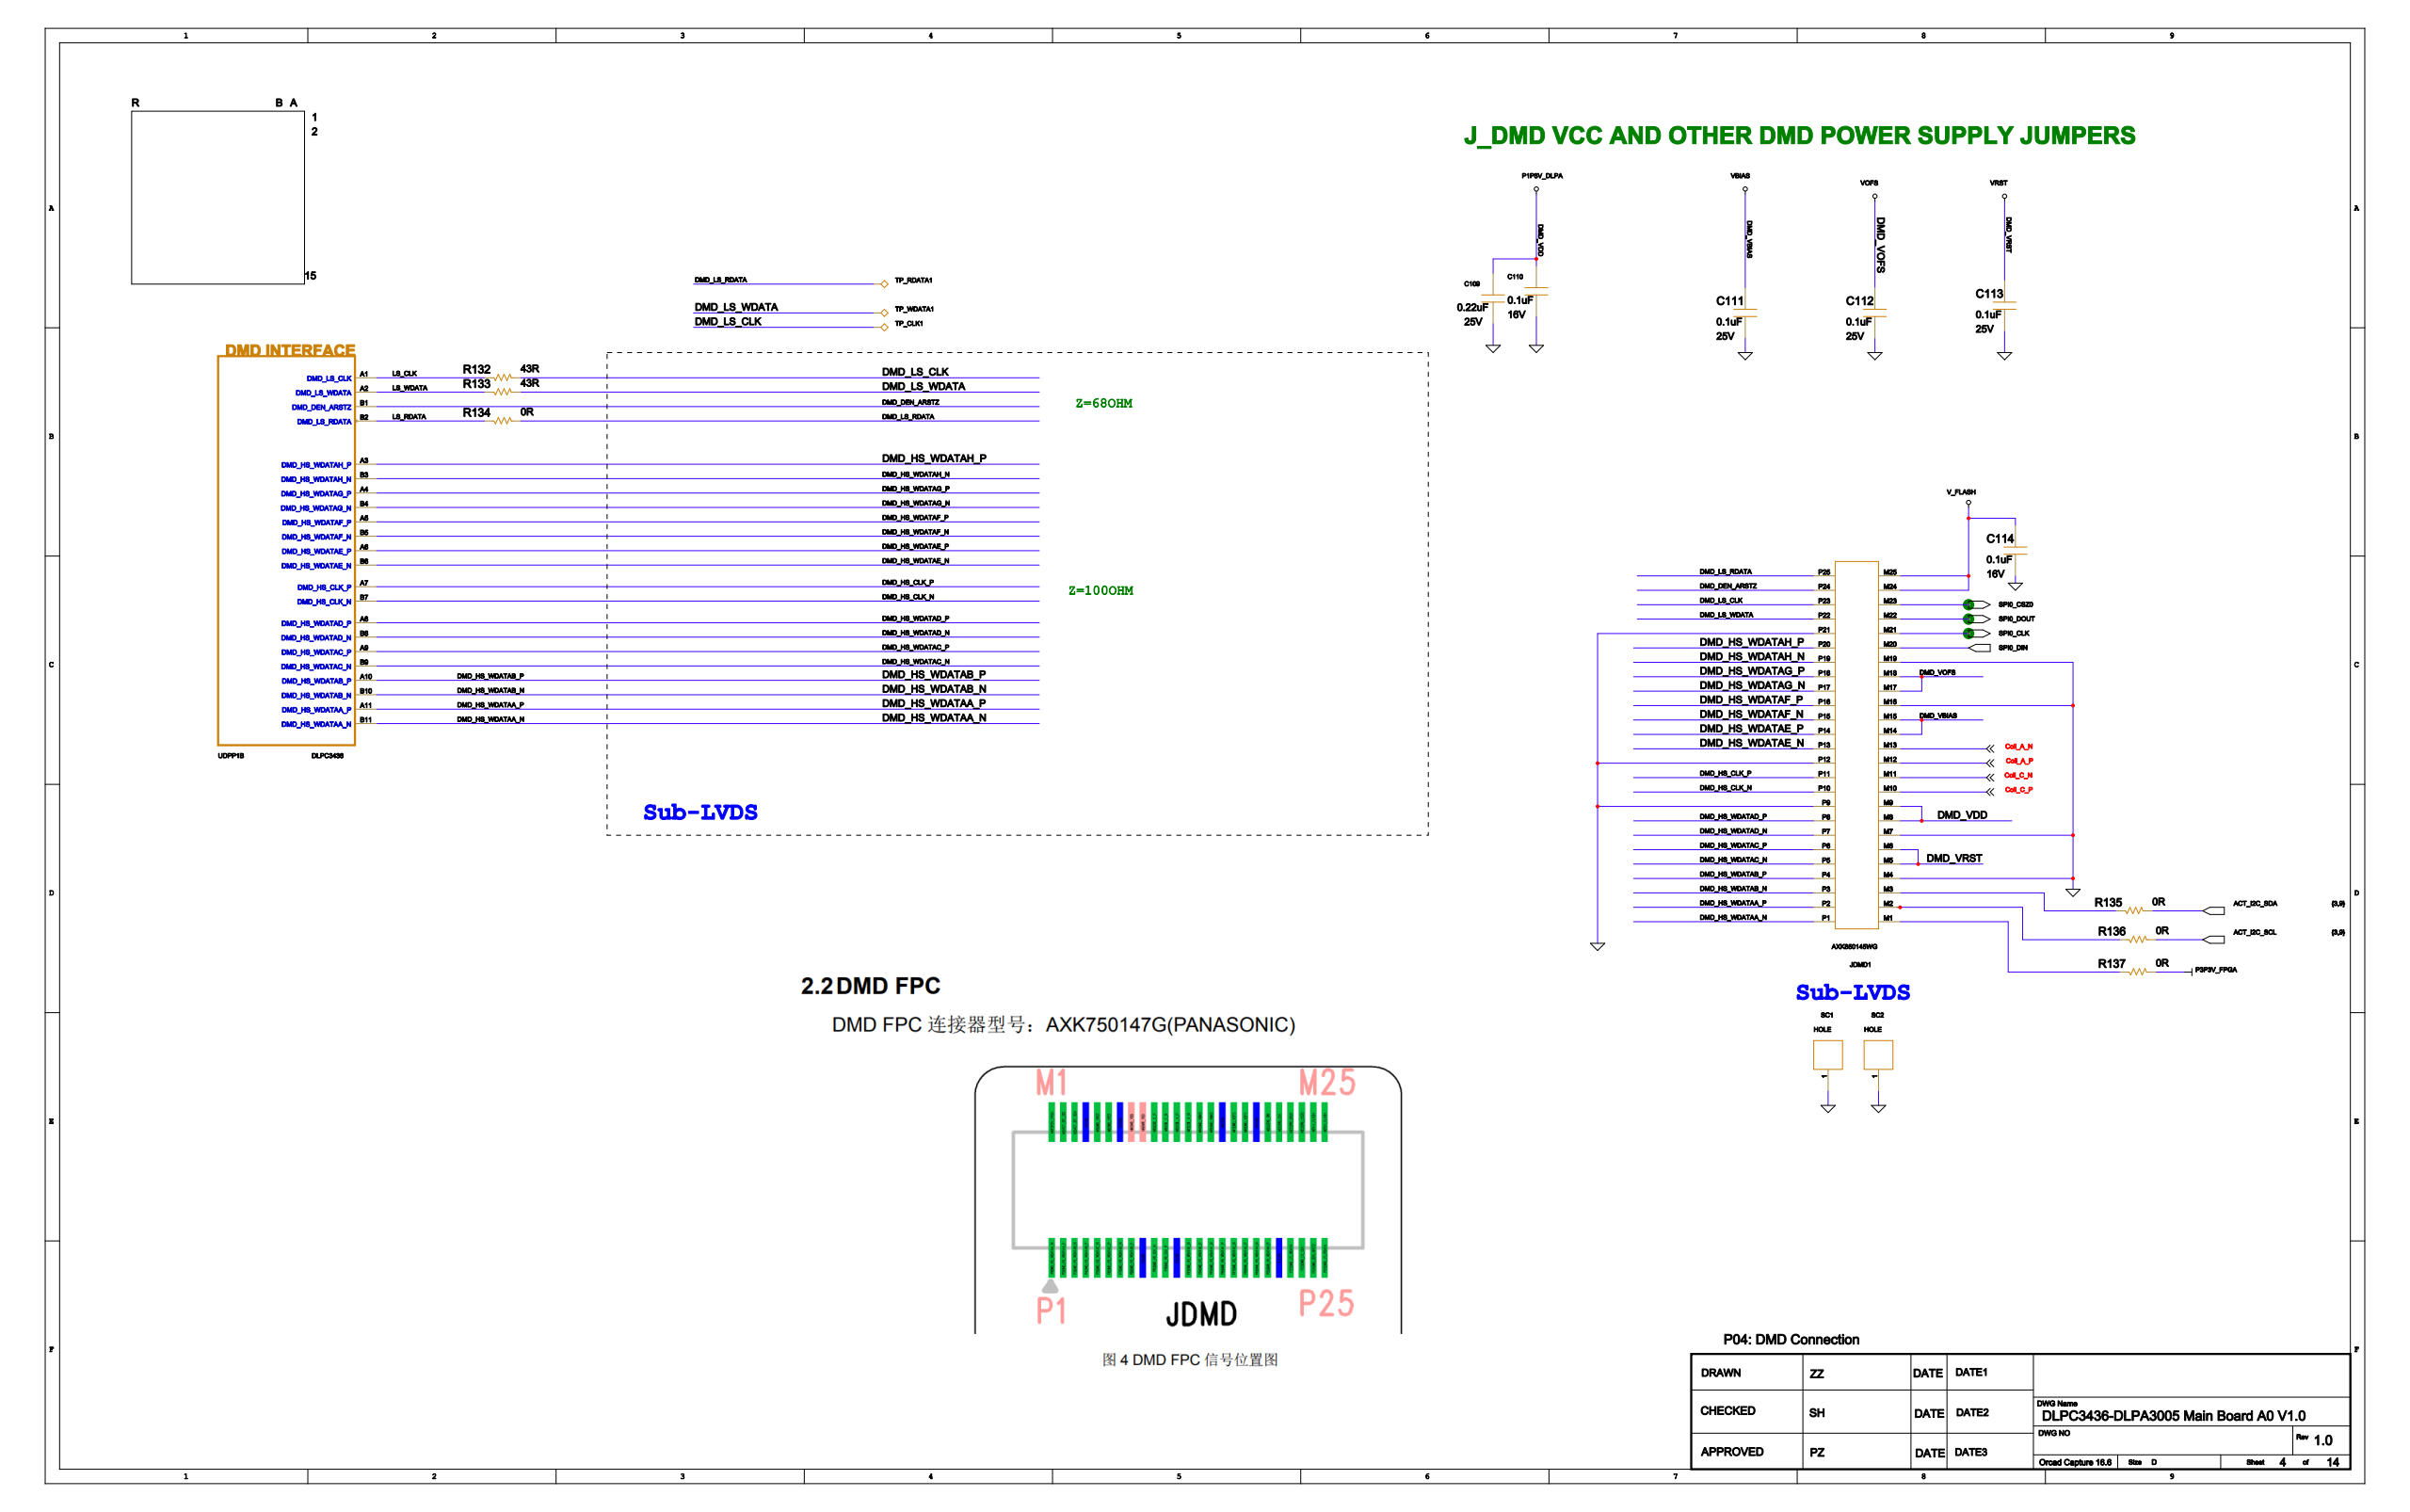Circuit board | Cadence Allegro | 1223 parts | 777 nets | one sheet of the schematic
Parts on this sheet (reference | value | footprint):
C109 | 0.22uF | C0402
C110 | 0.1uF | C0201
C111 | 0.1uF | C0402
C112 | 0.1uF | C0402
C113 | 0.1uF | C0402
C114 | 0.1uF | C0201
JDMD1 | AXK850145WG | AXK850145WG
P2 | HDMI/90D | HDMI_A
R132 | 43R | R0201
R133 | 43R | R0201
R134 | 0R | R0201
R135 | 0R | R0201
R136 | 0R | R0201
R137 | 0R | R0201
SC1 | HOLE | MHC4_2D3MM
SC2 | HOLE | MHC4_2D3MM
TP_CLK1 | TP40 | TP06MM
TP_RDATA1 | TP40 | TP06MM
TP_WDATA1 | TP40 | TP06MM
UDPP1 | DLPC3436 | DLPC3436_176NFBGA
Nets of these parts (net: part-pin ...):
GND: C109-2 C110-2 C111-2 C112-2 C113-2 C114-2 SC1-1 SC2-1 JDMD1-M4 JDMD1-M7 JDMD1-M16 JDMD1-M19 JDMD1-P9 JDMD1-P12 JDMD1-P21 P2-2 P2-5 P2-8 UDPP1-M4 UDPP1-M5 UDPP1-M8 UDPP1-M12
P3P3V_FPGA: R137-1
P1P8V_DLPA: C109-1 C110-1 JDMD1-M8 JDMD1-M9 UDPP1-M3 UDPP1-M7 UDPP1-M11
V_FLASH: C114-1 JDMD1-M24 JDMD1-M25
VBIAS: C111-1 JDMD1-M14 JDMD1-M15
VOFS: C112-1 JDMD1-M17 JDMD1-M18
VRST: C113-1 JDMD1-M5 JDMD1-M6
DMD_LS_CLK: R132-1 TP_CLK1-1 JDMD1-P23
DMD_LS_RDATA: R134-1 TP_RDATA1-1 JDMD1-P25
DMD_LS_WDATA: R133-1 TP_WDATA1-1 JDMD1-P22
ACT_I2C_SCL: R136-1
ACT_I2C_SDA: R135-1
N23995540: R137-2 JDMD1-M1
N23995448: R136-2 JDMD1-M2
SPI0_DIN: JDMD1-M20
SPI0_CLK: JDMD1-M21
SPI0_DOUT: JDMD1-M22
SPI0_CSZ0: JDMD1-M23
N23995520: R135-2 JDMD1-M3
DMD_HS_WDATAA_N: JDMD1-P1 UDPP1-B11
DMD_HS_CLK_N: JDMD1-P10 UDPP1-B7
DMD_HS_CLK_P: JDMD1-P11 UDPP1-A7
DMD_HS_WDATAE_N: JDMD1-P13 UDPP1-B6
DMD_HS_WDATAE_P: JDMD1-P14 UDPP1-A6
DMD_HS_WDATAF_N: JDMD1-P15 UDPP1-B5
DMD_HS_WDATAF_P: JDMD1-P16 UDPP1-A5
DMD_HS_WDATAG_N: JDMD1-P17 UDPP1-B4
DMD_HS_WDATAG_P: JDMD1-P18 UDPP1-A4
DMD_HS_WDATAH_N: JDMD1-P19 UDPP1-B3
DMD_HS_WDATAA_P: JDMD1-P2 UDPP1-A11
DMD_HS_WDATAH_P: JDMD1-P20 UDPP1-A3
DMD_DEN_ARSTZ: JDMD1-P24 UDPP1-B1
DMD_HS_WDATAB_N: JDMD1-P3 UDPP1-B10
DMD_HS_WDATAB_P: JDMD1-P4 UDPP1-A10
DMD_HS_WDATAC_N: JDMD1-P5 UDPP1-B9
DMD_HS_WDATAC_P: JDMD1-P6 UDPP1-A9
DMD_HS_WDATAD_N: JDMD1-P7 UDPP1-B8
DMD_HS_WDATAD_P: JDMD1-P8 UDPP1-A8
LS_RDATA: R134-2 UDPP1-B2
LS_CLK: R132-2 UDPP1-A1
LS_WDATA: R133-2 UDPP1-A2